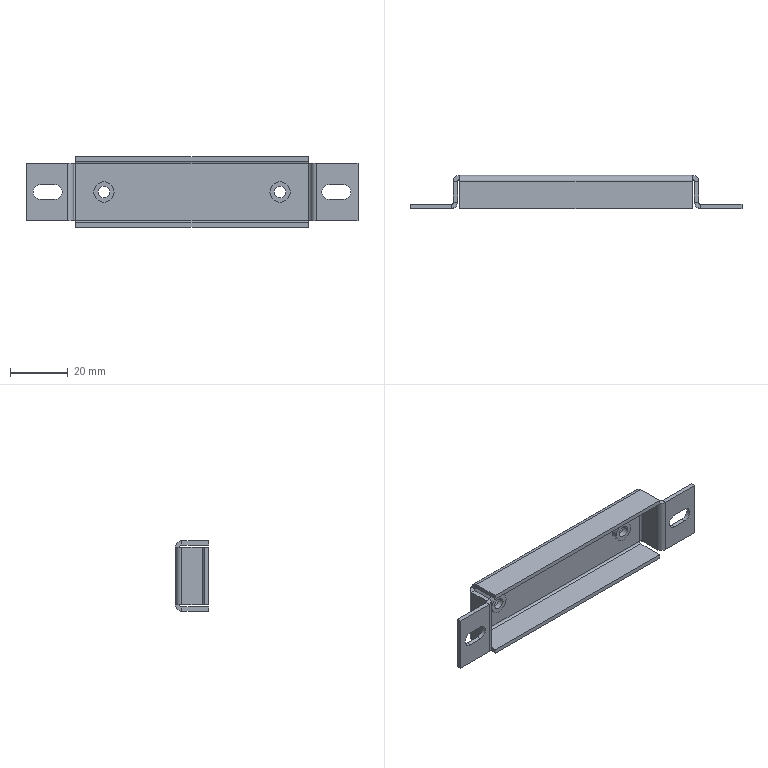Part | STEP file | FBDS-BJ-021 | 1 solid | 78 faces | box 115 x 11.5 x 24.473 mm | volume 6686 mm3 | plane 50 | cylinder 28 | commonest cylinder face diameters 5 x8 1.473 x6 4.473 x6 4 x4 7 x4